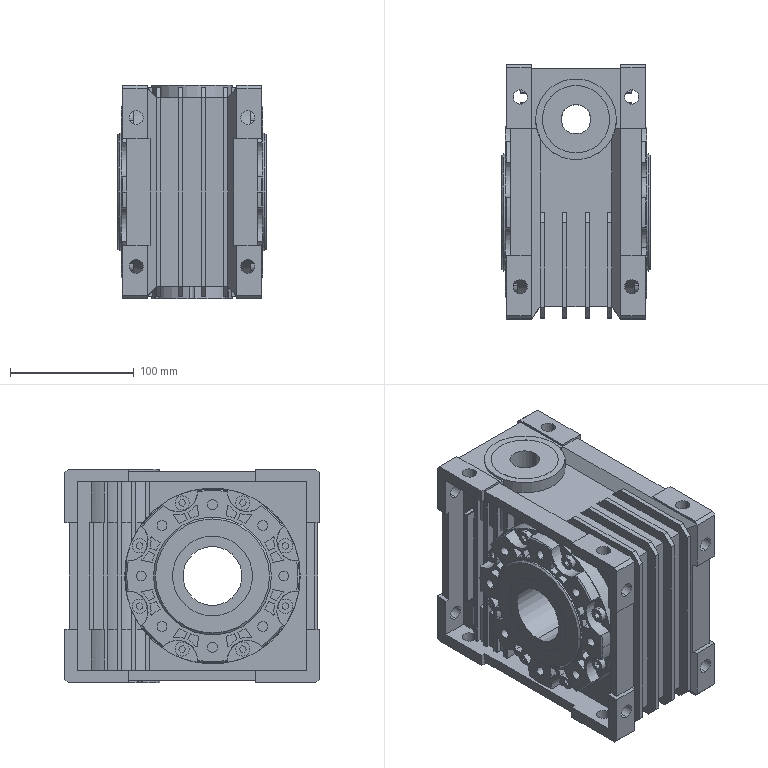Part | SolidWorks | features BaseBody 1, HoleWzd 1 | 1 solid | 857 faces | box 120 x 205 x 172 mm | volume 2864406 mm3 | plane 469 | cylinder 352 | cone 36 | commonest cylinder face diameters 1 x80 11.5 x64 36.765 x36 8 x32 99.75 x32 32.015 x24